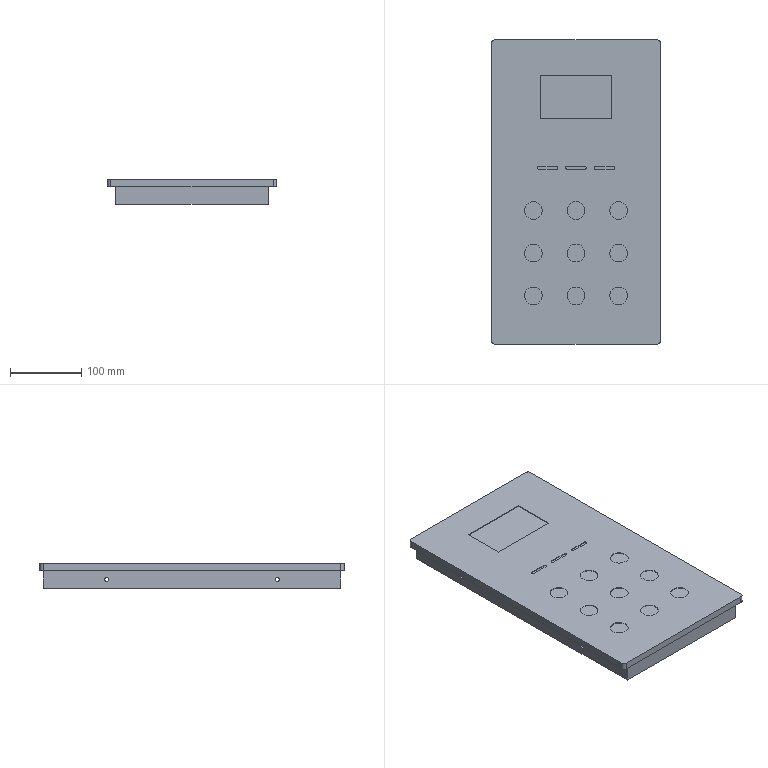Part | SolidWorks | features ICE 3, Extrusion 1, MoveCopyBody 1 | 1 solid | 69 faces | box 238 x 428 x 35 mm | volume 3242262 mm3 | cylinder 35 | plane 34 | commonest cylinder face diameters 25 x18 4 x9 6 x4 10 x4